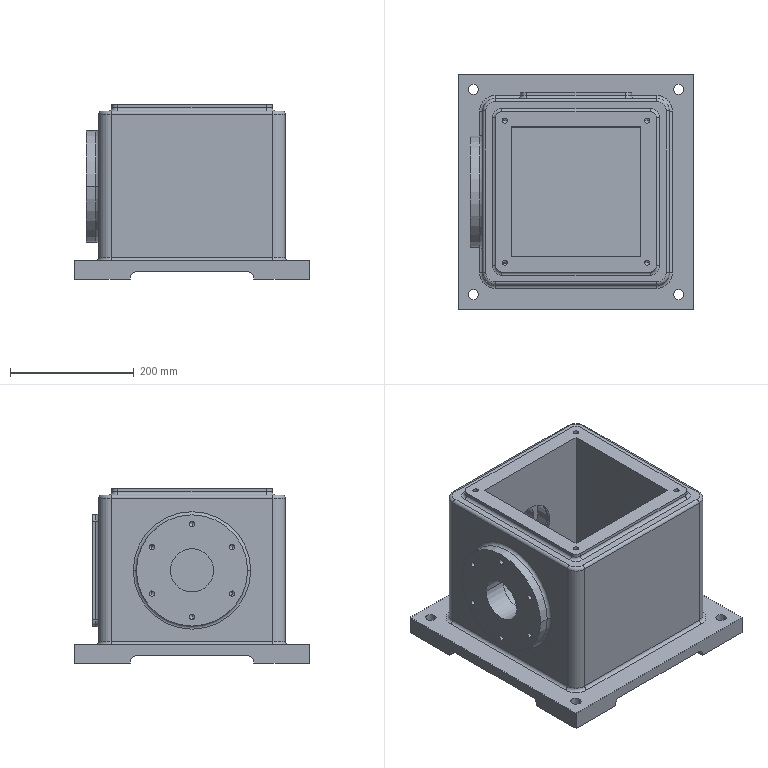Part | SolidWorks | features ICE 13, 3DProfileFeature 3, HoleWzd 3, Fillet 2, Extrusion 1 | 1 solid | 181 faces | box 380 x 380 x 282 mm | volume 14746846 mm3 | cylinder 90 | plane 45 | cone 28 | torus 18 | commonest cylinder face diameters 8.5 x28 10 x16 20 x16 16.5 x8 90 x8 40 x4